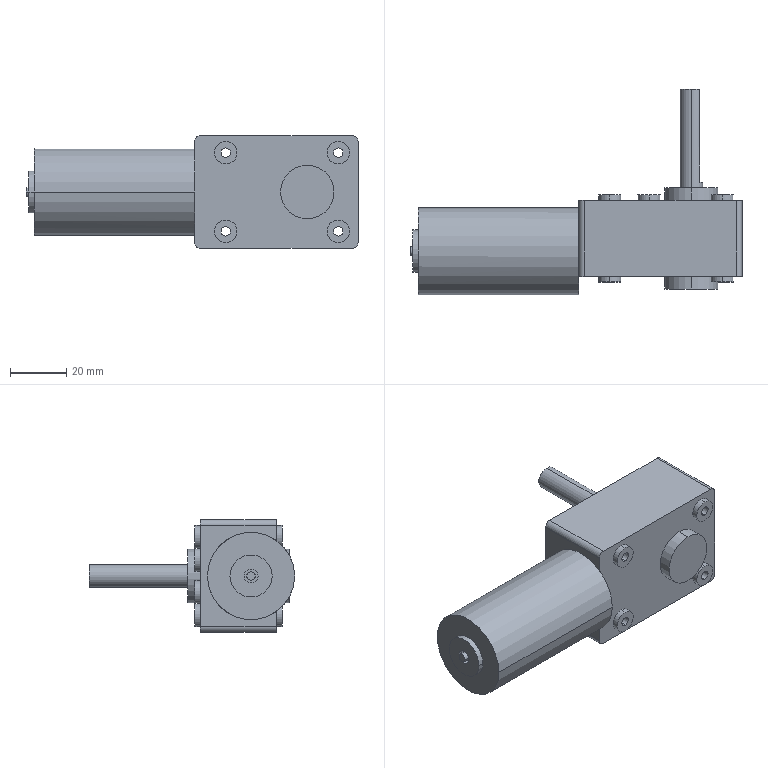Part | SolidWorks | features BaseBody 2 | 2 solids | 76 faces | box 118 x 73 x 40 mm | volume 109791 mm3 | cylinder 48 | plane 28 | commonest cylinder face diameters 8 x22 3.3 x8 4 x4 19 x4 3 x2 5 x2